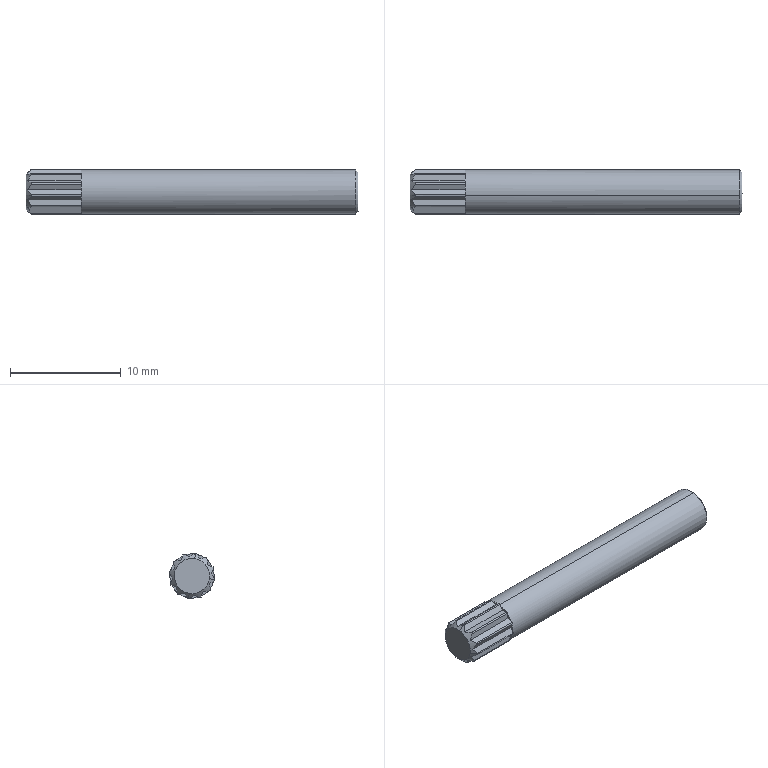Part | SolidWorks | features BaseBody 1 | 1 solid | 70 faces | box 30 x 4.153 x 4.153 mm | volume 371.268 mm3 | plane 50 | cylinder 14 | cone 6 | commonest cylinder face diameters 0.2 x12 4 x2